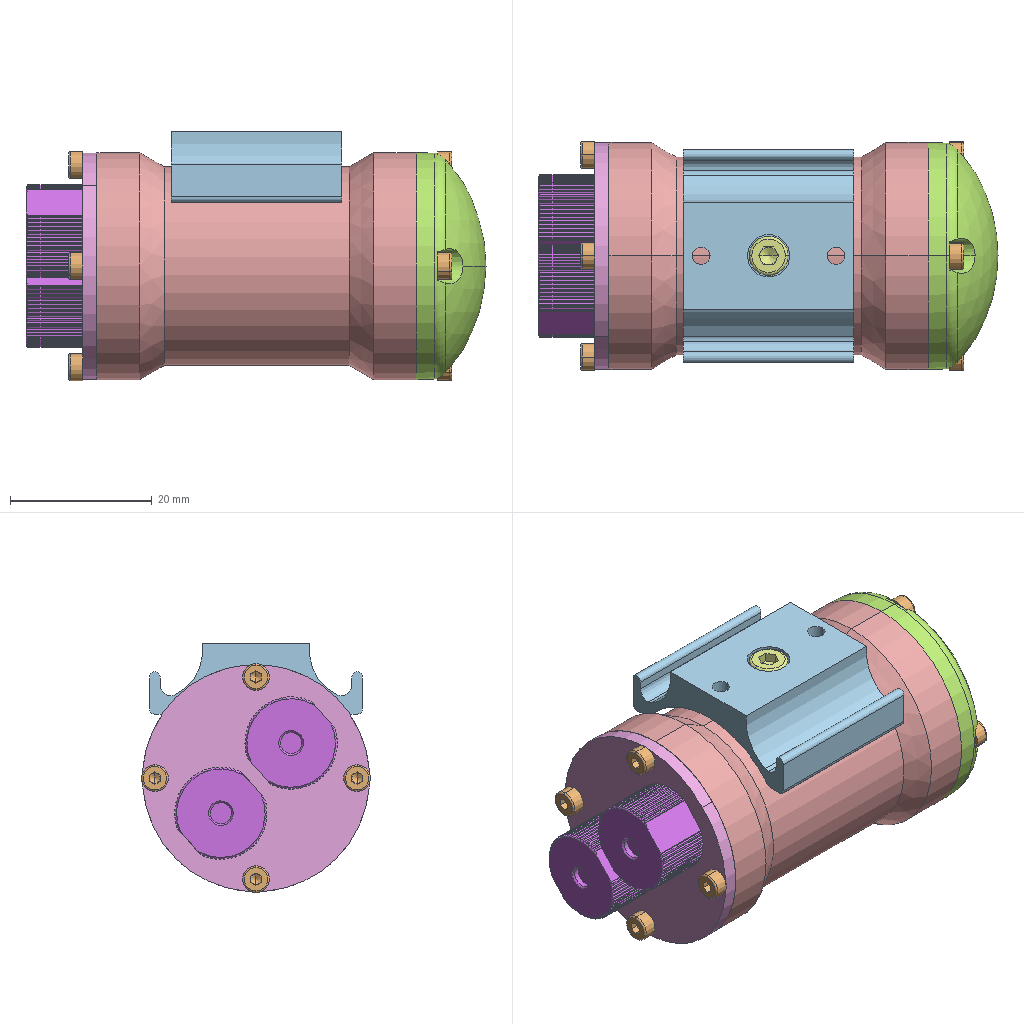Assembly | SolidWorks | 10 different items | 12 placed | box 65 x 32 x 35 mm
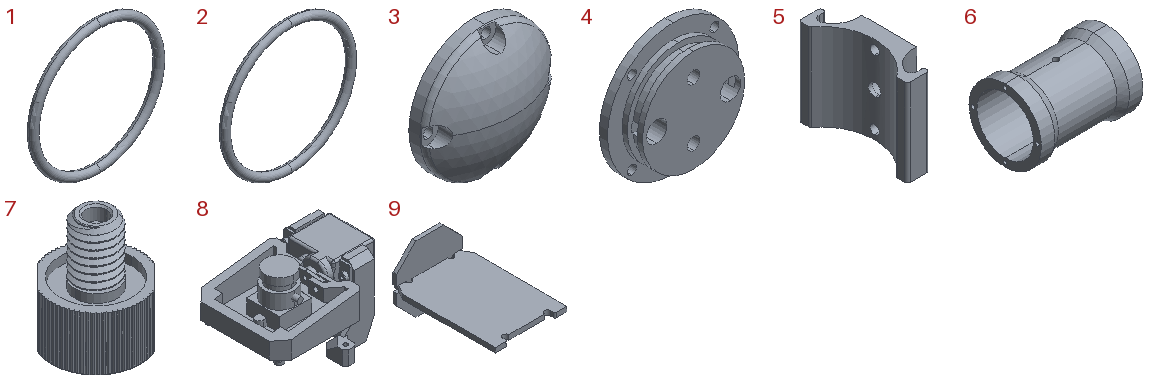Parts list (item | name | quantity | size | volume | features):
1 | - | x1 | 24 x 1.5 x 24 mm | 124.912 mm3 | features Revolution 1
2 | - | x2 | 25 x 1.5 x 25 mm | 130.464 mm3 | features Revolution 1
3 | - | x1 | 32 x 9.828 x 32 mm | 4397 mm3 | features HoleWzd 1, Revolution 1
4 | - | x1 | 32 x 7 x 32 mm | 3489 mm3 | features ICE 2, HoleWzd 1, Revolution 1
5 | - | x1 | 10 x 30 x 24 mm | 2596 mm3 | features HoleWzd 2, Extrusion 1
6 | - | x1 | 45.002 x 32 x 32 mm | 10043 mm3 | features HoleWzd 2, ICE 1, Revolution 1
7 | - | x2 | 13 x 13 x 16 mm | 1107 mm3 | features ICE 51, HoleWzd 2, BaseBody 1, Chamfer 1
8 | - | x1 | 62.8 x 44.75 x 40.65 mm | 30642 mm3 | features BaseBody 12
9 | - | x1 | 24 x 38.2 x 22.173 mm | 1798 mm3 | features ICE 2, Extrusion 1, Revolution 1
10 | hexagon socket head cap screws gb | x1 | - | - | -
Mates (type | each side: item.copy, entity, surface, feature):
Concentric | 6.1 face cylinder Revolve1 | 1.1 select_type:24
Tangent | 6.1 face plane Revolve1 | 1.1 face torus Revolve1
Concentric | 6.1 face cylinder Revolve1 | 3.1 face cone Revolve1
Coincident | 6.1 face plane Revolve1 | 3.1 face plane Revolve1
Coincident | 3.1 plane | assembly plane
Concentric | 6.1 face cylinder Revolve1 | 4.1 face cylinder Revolve1
Concentric | 4.1 face cylinder Revolve1 | 2.1 select_type:24
Tangent | 4.1 face plane Revolve1 | 2.1 face torus Revolve1
Concentric | 4.1 face cylinder Revolve1 | 2.2 select_type:24
Tangent | 4.1 face plane Revolve1 | 2.2 face torus Revolve1
Coincident | 6.1 face plane Revolve1 | 4.1 face plane Revolve1
Concentric | 6.1 face cylinder M2 Tapped Hole2 | 4.1 face cylinder Size mm Dowel Pin Hole1
Coincident | 6.1 edge | 9.1 face plane Boss-Extrude2
Coincident | 9.1 face plane Boss-Extrude1 | assembly plane
Symmetric | 9.1 face plane Boss-Extrude2 | 9.1 face plane Boss-Extrude2 | assembly plane
Concentric | 6.1 face cylinder Revolve1 | 5.1 face cylinder Boss-Extrude1
Symmetric | 6.1 plane | 5.1 face plane Boss-Extrude1 | 5.1 face plane Boss-Extrude1
Concentric | 6.1 face cylinder Cut-Extrude1 | 5.1 face cylinder Hole Size (% based on hex head bolt) Full thread type1
Concentric | 4.1 face cylinder Cut-Extrude1 | 7.1 face cylinder Cut-Extrude1
Coincident | 4.1 face plane Revolve1 | 7.1 face plane Input3
Concentric | 4.1 face cylinder Cut-Extrude1 | 7.2 face cylinder Cut-Extrude1